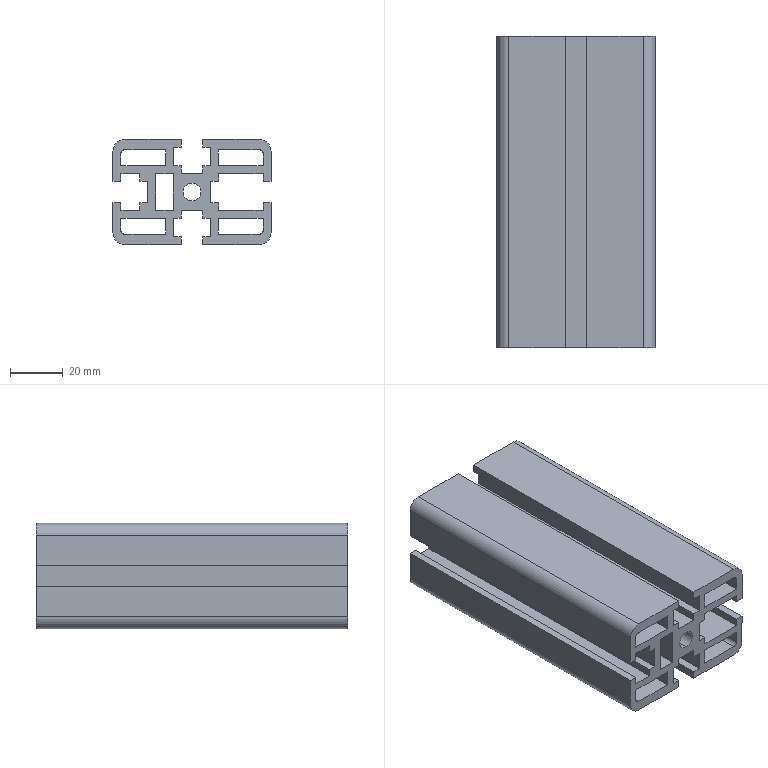Part | STEP file | Station 3 support_Default<machined> | 1 solid | 84 faces | box 60 x 118.295 x 40 mm | volume 132045 mm3 | plane 74 | cylinder 10 | commonest cylinder face diameters 3 x4 9 x4 6.8 x2